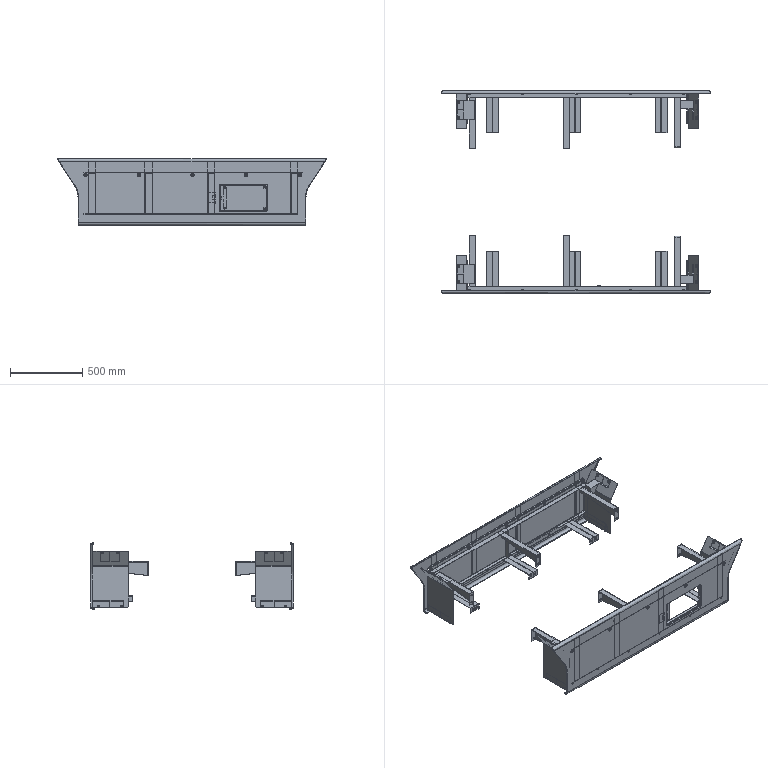Part | NX | features BREP 109 | 71 solids | 2521 faces | box 1856 x 1400 x 457 mm | volume 7771969 mm3 | plane 1469 | cylinder 752 | cone 228 | spline 50 | torus 22 | commonest cylinder face diameters 12 x108 11 x104 9 x92 13 x92 8 x80 10 x78